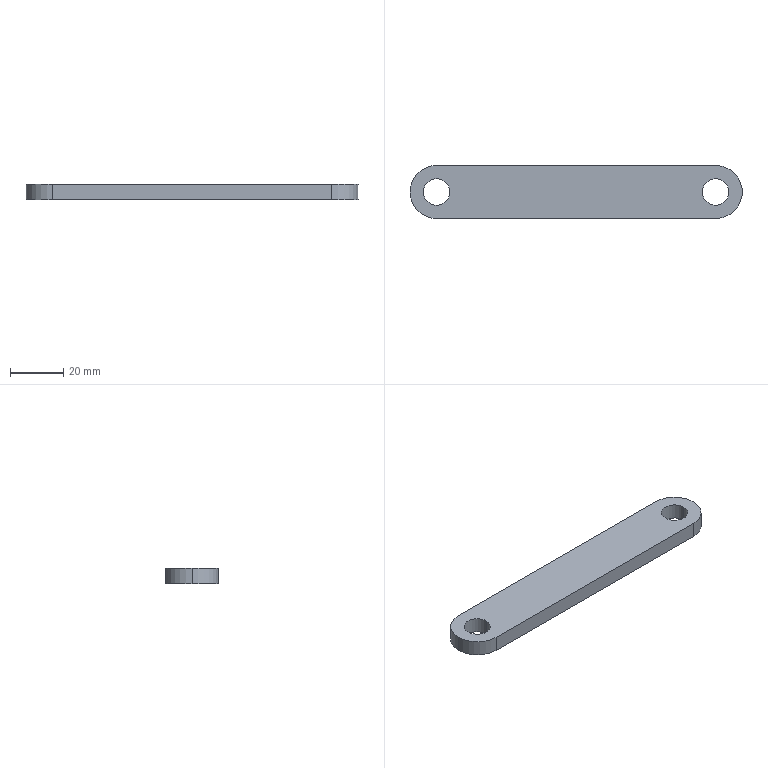Part | SolidWorks | features Extrusion 1 | 1 solid | 11 faces | box 125 x 20 x 6 mm | volume 13542 mm3 | cylinder 7 | plane 4 | commonest cylinder face diameters 10 x4 20 x3
STEP:
#1=CARTESIAN_POINT('',(100.,0.,3.));
#2=VERTEX_POINT('',#1);
#3=CARTESIAN_POINT('',(110.,0.,3.));
#4=VERTEX_POINT('',#3);
#5=CARTESIAN_POINT('',(105.,0.,3.));
#6=DIRECTION('',(0.,0.,1.));
#7=DIRECTION('',(1.,0.,0.));
#8=AXIS2_PLACEMENT_3D('',#5,#6,#7);
#9=CIRCLE('',#8,5.);
#10=EDGE_CURVE('',#2,#4,#9,.T.);
#11=ORIENTED_EDGE('',*,*,#10,.T.);
#12=CARTESIAN_POINT('',(110.,0.,-3.));
#13=VERTEX_POINT('',#12);
#14=CARTESIAN_POINT('',(110.,0.,3.));
#15=DIRECTION('',(0.,0.,-1.));
#16=VECTOR('',#15,1000.);
#17=LINE('',#14,#16);
#18=EDGE_CURVE('',#4,#13,#17,.T.);
#19=ORIENTED_EDGE('',*,*,#18,.T.);
#20=CARTESIAN_POINT('',(100.,0.,-3.));
#21=VERTEX_POINT('',#20);
#22=CARTESIAN_POINT('',(105.,0.,-3.));
#23=DIRECTION('',(0.,0.,1.));
#24=DIRECTION('',(1.,0.,0.));
#25=AXIS2_PLACEMENT_3D('',#22,#23,#24);
#26=CIRCLE('',#25,5.);
#27=EDGE_CURVE('',#21,#13,#26,.T.);
#28=ORIENTED_EDGE('',*,*,#27,.F.);
#29=CARTESIAN_POINT('',(100.,0.,3.));
#30=DIRECTION('',(0.,0.,-1.));
#31=VECTOR('',#30,1000.);
#32=LINE('',#29,#31);
#33=EDGE_CURVE('',#2,#21,#32,.T.);
#34=ORIENTED_EDGE('',*,*,#33,.F.);
#35=EDGE_LOOP('',(#11,#19,#28,#34));
#36=FACE_OUTER_BOUND('',#35,.T.);
#37=CARTESIAN_POINT('',(105.,0.,3.));
#38=DIRECTION('',(0.,0.,-1.));
#39=DIRECTION('',(-1.,0.,0.));
#40=AXIS2_PLACEMENT_3D('',#37,#38,#39);
#41=CYLINDRICAL_SURFACE('',#40,5.);
#42=ADVANCED_FACE('',(#36),#41,.F.);
#43=CARTESIAN_POINT('',(-5.,0.,3.));
#44=VERTEX_POINT('',#43);
#45=CARTESIAN_POINT('',(5.,0.,3.));
#46=VERTEX_POINT('',#45);
#47=CARTESIAN_POINT('',(0.,0.,3.));
#48=DIRECTION('',(0.,0.,1.));
#49=DIRECTION('',(1.,0.,0.));
#50=AXIS2_PLACEMENT_3D('',#47,#48,#49);
#51=CIRCLE('',#50,5.);
#52=EDGE_CURVE('',#44,#46,#51,.T.);
#53=ORIENTED_EDGE('',*,*,#52,.T.);
#54=CARTESIAN_POINT('',(5.,0.,-3.));
#55=VERTEX_POINT('',#54);
#56=CARTESIAN_POINT('',(5.,0.,3.));
#57=DIRECTION('',(0.,0.,-1.));
#58=VECTOR('',#57,1000.);
#59=LINE('',#56,#58);
#60=EDGE_CURVE('',#46,#55,#59,.T.);
#61=ORIENTED_EDGE('',*,*,#60,.T.);
#62=CARTESIAN_POINT('',(-5.,0.,-3.));
#63=VERTEX_POINT('',#62);
#64=CARTESIAN_POINT('',(0.,0.,-3.));
#65=DIRECTION('',(0.,0.,1.));
#66=DIRECTION('',(1.,0.,0.));
#67=AXIS2_PLACEMENT_3D('',#64,#65,#66);
#68=CIRCLE('',#67,5.);
#69=EDGE_CURVE('',#63,#55,#68,.T.);
#70=ORIENTED_EDGE('',*,*,#69,.F.);
#71=CARTESIAN_POINT('',(-5.,0.,3.));
#72=DIRECTION('',(0.,0.,-1.));
#73=VECTOR('',#72,1000.);
#74=LINE('',#71,#73);
#75=EDGE_CURVE('',#44,#63,#74,.T.);
#76=ORIENTED_EDGE('',*,*,#75,.F.);
#77=EDGE_LOOP('',(#53,#61,#70,#76));
#78=FACE_OUTER_BOUND('',#77,.T.);
#79=CARTESIAN_POINT('',(0.,0.,3.));
#80=DIRECTION('',(0.,0.,-1.));
#81=DIRECTION('',(-1.,0.,0.));
#82=AXIS2_PLACEMENT_3D('',#79,#80,#81);
#83=CYLINDRICAL_SURFACE('',#82,5.);
#84=ADVANCED_FACE('',(#78),#83,.F.);
#85=CARTESIAN_POINT('',(-10.,0.,3.));
#86=VERTEX_POINT('',#85);
#87=CARTESIAN_POINT('',(0.,-10.,3.));
#88=VERTEX_POINT('',#87);
#89=CARTESIAN_POINT('',(0.,0.,3.));
#90=DIRECTION('',(0.,0.,1.));
#91=DIRECTION('',(1.,0.,0.));
#92=AXIS2_PLACEMENT_3D('',#89,#90,#91);
#93=CIRCLE('',#92,10.);
#94=EDGE_CURVE('',#86,#88,#93,.T.);
#95=ORIENTED_EDGE('',*,*,#94,.F.);
#96=CARTESIAN_POINT('',(-10.,0.,-3.));
#97=VERTEX_POINT('',#96);
#98=CARTESIAN_POINT('',(-10.,0.,3.));
#99=DIRECTION('',(0.,0.,-1.));
#100=VECTOR('',#99,1000.);
#101=LINE('',#98,#100);
#102=EDGE_CURVE('',#86,#97,#101,.T.);
#103=ORIENTED_EDGE('',*,*,#102,.T.);
#104=CARTESIAN_POINT('',(0.,-10.,-3.));
#105=VERTEX_POINT('',#104);
#106=CARTESIAN_POINT('',(0.,0.,-3.));
#107=DIRECTION('',(0.,0.,1.));
#108=DIRECTION('',(1.,0.,0.));
#109=AXIS2_PLACEMENT_3D('',#106,#107,#108);
#110=CIRCLE('',#109,10.);
#111=EDGE_CURVE('',#97,#105,#110,.T.);
#112=ORIENTED_EDGE('',*,*,#111,.T.);
#113=CARTESIAN_POINT('',(0.,-10.,3.));
#114=DIRECTION('',(0.,0.,-1.));
#115=VECTOR('',#114,1000.);
#116=LINE('',#113,#115);
#117=EDGE_CURVE('',#88,#105,#116,.T.);
#118=ORIENTED_EDGE('',*,*,#117,.F.);
#119=EDGE_LOOP('',(#95,#103,#112,#118));
#120=FACE_OUTER_BOUND('',#119,.T.);
#121=CARTESIAN_POINT('',(0.,0.,3.));
#122=DIRECTION('',(0.,0.,-1.));
#123=DIRECTION('',(-1.,0.,0.));
#124=AXIS2_PLACEMENT_3D('',#121,#122,#123);
#125=CYLINDRICAL_SURFACE('',#124,10.);
#126=ADVANCED_FACE('',(#120),#125,.T.);
#127=ORIENTED_EDGE('',*,*,#52,.F.);
#128=CARTESIAN_POINT('',(0.,0.,3.));
#129=DIRECTION('',(0.,0.,1.));
#130=DIRECTION('',(1.,0.,0.));
#131=AXIS2_PLACEMENT_3D('',#128,#129,#130);
#132=CIRCLE('',#131,5.);
#133=EDGE_CURVE('',#46,#44,#132,.T.);
#134=ORIENTED_EDGE('',*,*,#133,.F.);
#135=EDGE_LOOP('',(#127,#134));
#136=FACE_BOUND('',#135,.T.);
#137=CARTESIAN_POINT('',(0.,10.,3.));
#138=VERTEX_POINT('',#137);
#139=CARTESIAN_POINT('',(0.,0.,3.));
#140=DIRECTION('',(0.,0.,1.));
#141=DIRECTION('',(1.,0.,0.));
#142=AXIS2_PLACEMENT_3D('',#139,#140,#141);
#143=CIRCLE('',#142,10.);
#144=EDGE_CURVE('',#138,#86,#143,.T.);
#145=ORIENTED_EDGE('',*,*,#144,.T.);
#146=ORIENTED_EDGE('',*,*,#94,.T.);
#147=CARTESIAN_POINT('',(105.,-10.,3.));
#148=VERTEX_POINT('',#147);
#149=CARTESIAN_POINT('',(0.,-10.,3.));
#150=DIRECTION('',(1.,0.,0.));
#151=VECTOR('',#150,1000.);
#152=LINE('',#149,#151);
#153=EDGE_CURVE('',#88,#148,#152,.T.);
#154=ORIENTED_EDGE('',*,*,#153,.T.);
#155=CARTESIAN_POINT('',(105.,10.,3.));
#156=VERTEX_POINT('',#155);
#157=CARTESIAN_POINT('',(105.,0.,3.));
#158=DIRECTION('',(0.,0.,1.));
#159=DIRECTION('',(1.,0.,0.));
#160=AXIS2_PLACEMENT_3D('',#157,#158,#159);
#161=CIRCLE('',#160,10.);
#162=EDGE_CURVE('',#148,#156,#161,.T.);
#163=ORIENTED_EDGE('',*,*,#162,.T.);
#164=CARTESIAN_POINT('',(0.,10.,3.));
#165=DIRECTION('',(-1.,0.,0.));
#166=VECTOR('',#165,1000.);
#167=LINE('',#164,#166);
#168=EDGE_CURVE('',#156,#138,#167,.T.);
#169=ORIENTED_EDGE('',*,*,#168,.T.);
#170=EDGE_LOOP('',(#145,#146,#154,#163,#169));
#171=FACE_OUTER_BOUND('',#170,.T.);
#172=ORIENTED_EDGE('',*,*,#10,.F.);
#173=CARTESIAN_POINT('',(105.,0.,3.));
#174=DIRECTION('',(0.,0.,1.));
#175=DIRECTION('',(1.,0.,0.));
#176=AXIS2_PLACEMENT_3D('',#173,#174,#175);
#177=CIRCLE('',#176,5.);
#178=EDGE_CURVE('',#4,#2,#177,.T.);
#179=ORIENTED_EDGE('',*,*,#178,.F.);
#180=EDGE_LOOP('',(#172,#179));
#181=FACE_BOUND('',#180,.T.);
#182=CARTESIAN_POINT('',(0.,0.,3.));
#183=DIRECTION('',(0.,0.,1.));
#184=DIRECTION('',(1.,0.,0.));
#185=AXIS2_PLACEMENT_3D('',#182,#183,#184);
#186=PLANE('',#185);
#187=ADVANCED_FACE('',(#136,#171,#181),#186,.T.);
#188=CARTESIAN_POINT('',(0.,10.,-3.));
#189=VERTEX_POINT('',#188);
#190=CARTESIAN_POINT('',(0.,0.,-3.));
#191=DIRECTION('',(0.,0.,1.));
#192=DIRECTION('',(1.,0.,0.));
#193=AXIS2_PLACEMENT_3D('',#190,#191,#192);
#194=CIRCLE('',#193,10.);
#195=EDGE_CURVE('',#189,#97,#194,.T.);
#196=ORIENTED_EDGE('',*,*,#195,.F.);
#197=CARTESIAN_POINT('',(105.,10.,-3.));
#198=VERTEX_POINT('',#197);
#199=CARTESIAN_POINT('',(0.,10.,-3.));
#200=DIRECTION('',(-1.,0.,0.));
#201=VECTOR('',#200,1000.);
#202=LINE('',#199,#201);
#203=EDGE_CURVE('',#198,#189,#202,.T.);
#204=ORIENTED_EDGE('',*,*,#203,.F.);
#205=CARTESIAN_POINT('',(105.,-10.,-3.));
#206=VERTEX_POINT('',#205);
#207=CARTESIAN_POINT('',(105.,0.,-3.));
#208=DIRECTION('',(0.,0.,1.));
#209=DIRECTION('',(1.,0.,0.));
#210=AXIS2_PLACEMENT_3D('',#207,#208,#209);
#211=CIRCLE('',#210,10.);
#212=EDGE_CURVE('',#206,#198,#211,.T.);
#213=ORIENTED_EDGE('',*,*,#212,.F.);
#214=CARTESIAN_POINT('',(0.,-10.,-3.));
#215=DIRECTION('',(1.,0.,0.));
#216=VECTOR('',#215,1000.);
#217=LINE('',#214,#216);
#218=EDGE_CURVE('',#105,#206,#217,.T.);
#219=ORIENTED_EDGE('',*,*,#218,.F.);
#220=ORIENTED_EDGE('',*,*,#111,.F.);
#221=EDGE_LOOP('',(#196,#204,#213,#219,#220));
#222=FACE_OUTER_BOUND('',#221,.T.);
#223=ORIENTED_EDGE('',*,*,#69,.T.);
#224=CARTESIAN_POINT('',(0.,0.,-3.));
#225=DIRECTION('',(0.,0.,1.));
#226=DIRECTION('',(1.,0.,0.));
#227=AXIS2_PLACEMENT_3D('',#224,#225,#226);
#228=CIRCLE('',#227,5.);
#229=EDGE_CURVE('',#55,#63,#228,.T.);
#230=ORIENTED_EDGE('',*,*,#229,.T.);
#231=EDGE_LOOP('',(#223,#230));
#232=FACE_BOUND('',#231,.T.);
#233=ORIENTED_EDGE('',*,*,#27,.T.);
#234=CARTESIAN_POINT('',(105.,0.,-3.));
#235=DIRECTION('',(0.,0.,1.));
#236=DIRECTION('',(1.,0.,0.));
#237=AXIS2_PLACEMENT_3D('',#234,#235,#236);
#238=CIRCLE('',#237,5.);
#239=EDGE_CURVE('',#13,#21,#238,.T.);
#240=ORIENTED_EDGE('',*,*,#239,.T.);
#241=EDGE_LOOP('',(#233,#240));
#242=FACE_BOUND('',#241,.T.);
#243=CARTESIAN_POINT('',(0.,0.,-3.));
#244=DIRECTION('',(0.,0.,1.));
#245=DIRECTION('',(1.,0.,0.));
#246=AXIS2_PLACEMENT_3D('',#243,#244,#245);
#247=PLANE('',#246);
#248=ADVANCED_FACE('',(#222,#232,#242),#247,.F.);
#249=ORIENTED_EDGE('',*,*,#102,.F.);
#250=ORIENTED_EDGE('',*,*,#144,.F.);
#251=CARTESIAN_POINT('',(0.,10.,3.));
#252=DIRECTION('',(0.,0.,-1.));
#253=VECTOR('',#252,1000.);
#254=LINE('',#251,#253);
#255=EDGE_CURVE('',#138,#189,#254,.T.);
#256=ORIENTED_EDGE('',*,*,#255,.T.);
#257=ORIENTED_EDGE('',*,*,#195,.T.);
#258=EDGE_LOOP('',(#249,#250,#256,#257));
#259=FACE_OUTER_BOUND('',#258,.T.);
#260=CARTESIAN_POINT('',(0.,0.,3.));
#261=DIRECTION('',(0.,0.,-1.));
#262=DIRECTION('',(-1.,0.,0.));
#263=AXIS2_PLACEMENT_3D('',#260,#261,#262);
#264=CYLINDRICAL_SURFACE('',#263,10.);
#265=ADVANCED_FACE('',(#259),#264,.T.);
#266=ORIENTED_EDGE('',*,*,#218,.T.);
#267=CARTESIAN_POINT('',(105.,-10.,3.));
#268=DIRECTION('',(0.,0.,-1.));
#269=VECTOR('',#268,1000.);
#270=LINE('',#267,#269);
#271=EDGE_CURVE('',#148,#206,#270,.T.);
#272=ORIENTED_EDGE('',*,*,#271,.F.);
#273=ORIENTED_EDGE('',*,*,#153,.F.);
#274=ORIENTED_EDGE('',*,*,#117,.T.);
#275=EDGE_LOOP('',(#266,#272,#273,#274));
#276=FACE_OUTER_BOUND('',#275,.T.);
#277=CARTESIAN_POINT('',(0.,-10.,3.));
#278=DIRECTION('',(0.,1.,0.));
#279=DIRECTION('',(0.,0.,1.));
#280=AXIS2_PLACEMENT_3D('',#277,#278,#279);
#281=PLANE('',#280);
#282=ADVANCED_FACE('',(#276),#281,.F.);
#283=ORIENTED_EDGE('',*,*,#212,.T.);
#284=CARTESIAN_POINT('',(105.,10.,3.));
#285=DIRECTION('',(0.,0.,-1.));
#286=VECTOR('',#285,1000.);
#287=LINE('',#284,#286);
#288=EDGE_CURVE('',#156,#198,#287,.T.);
#289=ORIENTED_EDGE('',*,*,#288,.F.);
#290=ORIENTED_EDGE('',*,*,#162,.F.);
#291=ORIENTED_EDGE('',*,*,#271,.T.);
#292=EDGE_LOOP('',(#283,#289,#290,#291));
#293=FACE_OUTER_BOUND('',#292,.T.);
#294=CARTESIAN_POINT('',(105.,0.,3.));
#295=DIRECTION('',(0.,0.,-1.));
#296=DIRECTION('',(-1.,0.,0.));
#297=AXIS2_PLACEMENT_3D('',#294,#295,#296);
#298=CYLINDRICAL_SURFACE('',#297,10.);
#299=ADVANCED_FACE('',(#293),#298,.T.);
#300=ORIENTED_EDGE('',*,*,#203,.T.);
#301=ORIENTED_EDGE('',*,*,#255,.F.);
#302=ORIENTED_EDGE('',*,*,#168,.F.);
#303=ORIENTED_EDGE('',*,*,#288,.T.);
#304=EDGE_LOOP('',(#300,#301,#302,#303));
#305=FACE_OUTER_BOUND('',#304,.T.);
#306=CARTESIAN_POINT('',(0.,10.,3.));
#307=DIRECTION('',(0.,-1.,0.));
#308=DIRECTION('',(0.,0.,-1.));
#309=AXIS2_PLACEMENT_3D('',#306,#307,#308);
#310=PLANE('',#309);
#311=ADVANCED_FACE('',(#305),#310,.F.);
#312=ORIENTED_EDGE('',*,*,#60,.F.);
#313=ORIENTED_EDGE('',*,*,#133,.T.);
#314=ORIENTED_EDGE('',*,*,#75,.T.);
#315=ORIENTED_EDGE('',*,*,#229,.F.);
#316=EDGE_LOOP('',(#312,#313,#314,#315));
#317=FACE_OUTER_BOUND('',#316,.T.);
#318=CARTESIAN_POINT('',(0.,0.,3.));
#319=DIRECTION('',(0.,0.,-1.));
#320=DIRECTION('',(-1.,0.,0.));
#321=AXIS2_PLACEMENT_3D('',#318,#319,#320);
#322=CYLINDRICAL_SURFACE('',#321,5.);
#323=ADVANCED_FACE('',(#317),#322,.F.);
#324=ORIENTED_EDGE('',*,*,#18,.F.);
#325=ORIENTED_EDGE('',*,*,#178,.T.);
#326=ORIENTED_EDGE('',*,*,#33,.T.);
#327=ORIENTED_EDGE('',*,*,#239,.F.);
#328=EDGE_LOOP('',(#324,#325,#326,#327));
#329=FACE_OUTER_BOUND('',#328,.T.);
#330=CARTESIAN_POINT('',(105.,0.,3.));
#331=DIRECTION('',(0.,0.,-1.));
#332=DIRECTION('',(-1.,0.,0.));
#333=AXIS2_PLACEMENT_3D('',#330,#331,#332);
#334=CYLINDRICAL_SURFACE('',#333,5.);
#335=ADVANCED_FACE('',(#329),#334,.F.);
#336=CLOSED_SHELL('',(#42,#84,#126,#187,#248,#265,#282,#299,#311,#323,#335));
#337=MANIFOLD_SOLID_BREP('',#336);
#338=CARTESIAN_POINT('',(0.,0.,0.));
#339=DIRECTION('',(0.,0.,1.));
#340=DIRECTION('',(1.,0.,0.));
#341=AXIS2_PLACEMENT_3D('',#338,#339,#340);
#342=(LENGTH_UNIT()NAMED_UNIT(*)SI_UNIT(.MILLI.,.METRE.));
#343=UNCERTAINTY_MEASURE_WITH_UNIT(LENGTH_MEASURE(0.00001),#342,'','');
#344=(NAMED_UNIT(*)PLANE_ANGLE_UNIT()SI_UNIT($,.RADIAN.));
#345=(NAMED_UNIT(*)SI_UNIT($,.STERADIAN.)SOLID_ANGLE_UNIT());
#346=(GEOMETRIC_REPRESENTATION_CONTEXT(3)GLOBAL_UNCERTAINTY_ASSIGNED_CONTEXT((#343))GLOBAL_UNIT_ASSIGNED_CONTEXT((#342,#344,#345))REPRESENTATION_CONTEXT('',''));
#347=ADVANCED_BREP_SHAPE_REPRESENTATION('',(#337,#341),#346);